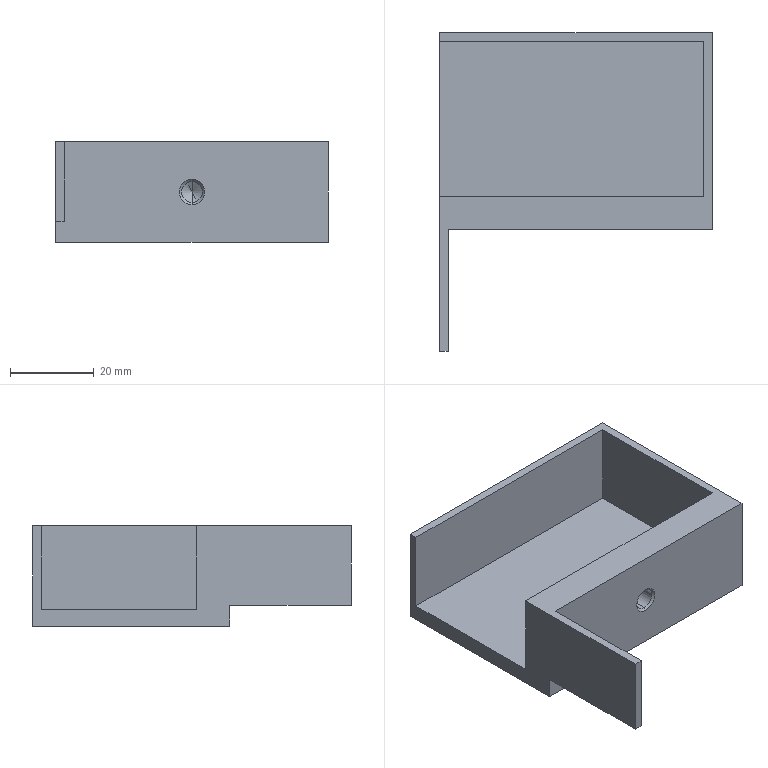Part | STEP file | 料槽1 | 1 solid | 19 faces | box 65 x 76 x 24 mm | volume 27672 mm3 | plane 13 | cone 4 | cylinder 2 | commonest cylinder face diameters 5 x2
STEP:
#1=CARTESIAN_POINT('',(159.5,-0.975,14.5));
#2=VERTEX_POINT('',#1);
#3=CARTESIAN_POINT('',(159.5,-0.975,9.5));
#4=VERTEX_POINT('',#3);
#5=CARTESIAN_POINT('',(159.5,-0.975,12.));
#6=DIRECTION('',(0.,-1.,0.));
#7=DIRECTION('',(0.,0.,-1.));
#8=AXIS2_PLACEMENT_3D('',#5,#6,#7);
#9=CIRCLE('',#8,2.5);
#10=EDGE_CURVE('',#2,#4,#9,.T.);
#11=ORIENTED_EDGE('',*,*,#10,.F.);
#12=CARTESIAN_POINT('',(159.5,-1.5,15.025));
#13=VERTEX_POINT('',#12);
#14=CARTESIAN_POINT('',(159.5,-1.5,15.025));
#15=DIRECTION('',(0.,-0.7071,0.7071));
#16=VECTOR('',#15,1000.);
#17=LINE('',#14,#16);
#18=EDGE_CURVE('',#2,#13,#17,.T.);
#19=ORIENTED_EDGE('',*,*,#18,.T.);
#20=CARTESIAN_POINT('',(159.5,-1.5,8.975));
#21=VERTEX_POINT('',#20);
#22=CARTESIAN_POINT('',(159.5,-1.5,12.));
#23=DIRECTION('',(0.,-1.,0.));
#24=DIRECTION('',(0.,0.,-1.));
#25=AXIS2_PLACEMENT_3D('',#22,#23,#24);
#26=CIRCLE('',#25,3.025);
#27=EDGE_CURVE('',#13,#21,#26,.T.);
#28=ORIENTED_EDGE('',*,*,#27,.T.);
#29=CARTESIAN_POINT('',(159.5,-1.5,8.975));
#30=DIRECTION('',(0.,-0.7071,-0.7071));
#31=VECTOR('',#30,1000.);
#32=LINE('',#29,#31);
#33=EDGE_CURVE('',#4,#21,#32,.T.);
#34=ORIENTED_EDGE('',*,*,#33,.F.);
#35=EDGE_LOOP('',(#11,#19,#28,#34));
#36=FACE_OUTER_BOUND('',#35,.T.);
#37=CARTESIAN_POINT('',(159.5,-1.5,12.));
#38=DIRECTION('',(0.,-1.,0.));
#39=DIRECTION('',(0.,0.,-1.));
#40=AXIS2_PLACEMENT_3D('',#37,#38,#39);
#41=CONICAL_SURFACE('',#40,3.025,0.7854);
#42=ADVANCED_FACE('',(#36),#41,.F.);
#43=CARTESIAN_POINT('',(159.5,4.5,14.5));
#44=VERTEX_POINT('',#43);
#45=CARTESIAN_POINT('',(159.5,4.5,9.5));
#46=VERTEX_POINT('',#45);
#47=CARTESIAN_POINT('',(159.5,4.5,12.));
#48=DIRECTION('',(0.,-1.,0.));
#49=DIRECTION('',(0.,0.,-1.));
#50=AXIS2_PLACEMENT_3D('',#47,#48,#49);
#51=CIRCLE('',#50,2.5);
#52=EDGE_CURVE('',#44,#46,#51,.T.);
#53=ORIENTED_EDGE('',*,*,#52,.F.);
#54=CARTESIAN_POINT('',(159.5,-1.5,14.5));
#55=DIRECTION('',(0.,-1.,0.));
#56=VECTOR('',#55,1000.);
#57=LINE('',#54,#56);
#58=EDGE_CURVE('',#44,#2,#57,.T.);
#59=ORIENTED_EDGE('',*,*,#58,.T.);
#60=ORIENTED_EDGE('',*,*,#10,.T.);
#61=CARTESIAN_POINT('',(159.5,-1.5,9.5));
#62=DIRECTION('',(0.,-1.,0.));
#63=VECTOR('',#62,1000.);
#64=LINE('',#61,#63);
#65=EDGE_CURVE('',#46,#4,#64,.T.);
#66=ORIENTED_EDGE('',*,*,#65,.F.);
#67=EDGE_LOOP('',(#53,#59,#60,#66));
#68=FACE_OUTER_BOUND('',#67,.T.);
#69=CARTESIAN_POINT('',(159.5,-1.5,12.));
#70=DIRECTION('',(0.,-1.,0.));
#71=DIRECTION('',(0.,0.,-1.));
#72=AXIS2_PLACEMENT_3D('',#69,#70,#71);
#73=CYLINDRICAL_SURFACE('',#72,2.5);
#74=ADVANCED_FACE('',(#68),#73,.F.);
#75=CARTESIAN_POINT('',(159.5,6.002,12.));
#76=VERTEX_POINT('',#75);
#77=CARTESIAN_POINT('',(159.5,4.5,9.5));
#78=DIRECTION('',(0.,-0.515,-0.8572));
#79=VECTOR('',#78,1000.);
#80=LINE('',#77,#79);
#81=EDGE_CURVE('',#76,#46,#80,.T.);
#82=ORIENTED_EDGE('',*,*,#81,.F.);
#83=CARTESIAN_POINT('',(159.5,4.5,14.5));
#84=DIRECTION('',(0.,-0.515,0.8572));
#85=VECTOR('',#84,1000.);
#86=LINE('',#83,#85);
#87=EDGE_CURVE('',#76,#44,#86,.T.);
#88=ORIENTED_EDGE('',*,*,#87,.T.);
#89=ORIENTED_EDGE('',*,*,#52,.T.);
#90=EDGE_LOOP('',(#82,#88,#89));
#91=FACE_OUTER_BOUND('',#90,.T.);
#92=CARTESIAN_POINT('',(159.5,4.5,12.));
#93=DIRECTION('',(0.,-1.,0.));
#94=DIRECTION('',(0.,0.,-1.));
#95=AXIS2_PLACEMENT_3D('',#92,#93,#94);
#96=CONICAL_SURFACE('',#95,2.5,1.03);
#97=ADVANCED_FACE('',(#91),#96,.F.);
#98=CARTESIAN_POINT('',(192.,45.5,0.));
#99=VERTEX_POINT('',#98);
#100=CARTESIAN_POINT('',(127.,45.5,0.));
#101=VERTEX_POINT('',#100);
#102=CARTESIAN_POINT('',(190.,45.5,0.));
#103=DIRECTION('',(-1.,0.,0.));
#104=VECTOR('',#103,1000.);
#105=LINE('',#102,#104);
#106=EDGE_CURVE('',#99,#101,#105,.T.);
#107=ORIENTED_EDGE('',*,*,#106,.T.);
#108=CARTESIAN_POINT('',(127.,45.5,24.));
#109=VERTEX_POINT('',#108);
#110=CARTESIAN_POINT('',(127.,45.5,4.));
#111=DIRECTION('',(0.,0.,-1.));
#112=VECTOR('',#111,1000.);
#113=LINE('',#110,#112);
#114=EDGE_CURVE('',#109,#101,#113,.T.);
#115=ORIENTED_EDGE('',*,*,#114,.F.);
#116=CARTESIAN_POINT('',(192.,45.5,24.));
#117=VERTEX_POINT('',#116);
#118=CARTESIAN_POINT('',(210.1,45.5,24.));
#119=DIRECTION('',(-1.,0.,0.));
#120=VECTOR('',#119,1000.);
#121=LINE('',#118,#120);
#122=EDGE_CURVE('',#117,#109,#121,.T.);
#123=ORIENTED_EDGE('',*,*,#122,.F.);
#124=CARTESIAN_POINT('',(192.,45.5,24.));
#125=DIRECTION('',(0.,0.,1.));
#126=VECTOR('',#125,1000.);
#127=LINE('',#124,#126);
#128=EDGE_CURVE('',#99,#117,#127,.T.);
#129=ORIENTED_EDGE('',*,*,#128,.F.);
#130=EDGE_LOOP('',(#107,#115,#123,#129));
#131=FACE_OUTER_BOUND('',#130,.T.);
#132=CARTESIAN_POINT('',(190.,45.5,4.));
#133=DIRECTION('',(0.,-1.,0.));
#134=DIRECTION('',(1.,0.,0.));
#135=AXIS2_PLACEMENT_3D('',#132,#133,#134);
#136=PLANE('',#135);
#137=ADVANCED_FACE('',(#131),#136,.F.);
#138=CARTESIAN_POINT('',(127.,-1.5,0.));
#139=VERTEX_POINT('',#138);
#140=CARTESIAN_POINT('',(127.,45.5,0.));
#141=DIRECTION('',(0.,-1.,0.));
#142=VECTOR('',#141,1000.);
#143=LINE('',#140,#142);
#144=EDGE_CURVE('',#101,#139,#143,.T.);
#145=ORIENTED_EDGE('',*,*,#144,.T.);
#146=CARTESIAN_POINT('',(127.,-1.5,5.));
#147=VERTEX_POINT('',#146);
#148=CARTESIAN_POINT('',(127.,-1.5,24.));
#149=DIRECTION('',(0.,0.,-1.));
#150=VECTOR('',#149,1000.);
#151=LINE('',#148,#150);
#152=EDGE_CURVE('',#147,#139,#151,.T.);
#153=ORIENTED_EDGE('',*,*,#152,.F.);
#154=CARTESIAN_POINT('',(127.,-30.5,5.));
#155=VERTEX_POINT('',#154);
#156=CARTESIAN_POINT('',(127.,-30.5,5.));
#157=DIRECTION('',(0.,1.,0.));
#158=VECTOR('',#157,1000.);
#159=LINE('',#156,#158);
#160=EDGE_CURVE('',#155,#147,#159,.T.);
#161=ORIENTED_EDGE('',*,*,#160,.F.);
#162=CARTESIAN_POINT('',(127.,-30.5,24.));
#163=VERTEX_POINT('',#162);
#164=CARTESIAN_POINT('',(127.,-30.5,24.));
#165=DIRECTION('',(0.,0.,-1.));
#166=VECTOR('',#165,1000.);
#167=LINE('',#164,#166);
#168=EDGE_CURVE('',#163,#155,#167,.T.);
#169=ORIENTED_EDGE('',*,*,#168,.F.);
#170=CARTESIAN_POINT('',(127.,6.5,24.));
#171=VERTEX_POINT('',#170);
#172=CARTESIAN_POINT('',(127.,4.5,24.));
#173=DIRECTION('',(0.,1.,0.));
#174=VECTOR('',#173,1000.);
#175=LINE('',#172,#174);
#176=EDGE_CURVE('',#163,#171,#175,.T.);
#177=ORIENTED_EDGE('',*,*,#176,.T.);
#178=CARTESIAN_POINT('',(127.,6.5,4.));
#179=VERTEX_POINT('',#178);
#180=CARTESIAN_POINT('',(127.,6.5,24.));
#181=DIRECTION('',(0.,0.,-1.));
#182=VECTOR('',#181,1000.);
#183=LINE('',#180,#182);
#184=EDGE_CURVE('',#171,#179,#183,.T.);
#185=ORIENTED_EDGE('',*,*,#184,.T.);
#186=CARTESIAN_POINT('',(127.,43.5,4.));
#187=VERTEX_POINT('',#186);
#188=CARTESIAN_POINT('',(127.,45.5,4.));
#189=DIRECTION('',(0.,-1.,0.));
#190=VECTOR('',#189,1000.);
#191=LINE('',#188,#190);
#192=EDGE_CURVE('',#187,#179,#191,.T.);
#193=ORIENTED_EDGE('',*,*,#192,.F.);
#194=CARTESIAN_POINT('',(127.,43.5,24.));
#195=VERTEX_POINT('',#194);
#196=CARTESIAN_POINT('',(127.,43.5,24.));
#197=DIRECTION('',(0.,0.,1.));
#198=VECTOR('',#197,1000.);
#199=LINE('',#196,#198);
#200=EDGE_CURVE('',#187,#195,#199,.T.);
#201=ORIENTED_EDGE('',*,*,#200,.T.);
#202=CARTESIAN_POINT('',(127.,45.5,24.));
#203=DIRECTION('',(0.,1.,0.));
#204=VECTOR('',#203,1000.);
#205=LINE('',#202,#204);
#206=EDGE_CURVE('',#195,#109,#205,.T.);
#207=ORIENTED_EDGE('',*,*,#206,.T.);
#208=ORIENTED_EDGE('',*,*,#114,.T.);
#209=EDGE_LOOP('',(#145,#153,#161,#169,#177,#185,#193,#201,#207,#208));
#210=FACE_OUTER_BOUND('',#209,.T.);
#211=CARTESIAN_POINT('',(127.,45.5,4.));
#212=DIRECTION('',(1.,0.,0.));
#213=DIRECTION('',(0.,0.,-1.));
#214=AXIS2_PLACEMENT_3D('',#211,#212,#213);
#215=PLANE('',#214);
#216=ADVANCED_FACE('',(#210),#215,.F.);
#217=ORIENTED_EDGE('',*,*,#192,.T.);
#218=CARTESIAN_POINT('',(190.,6.5,4.));
#219=VERTEX_POINT('',#218);
#220=CARTESIAN_POINT('',(210.1,6.5,4.));
#221=DIRECTION('',(-1.,0.,0.));
#222=VECTOR('',#221,1000.);
#223=LINE('',#220,#222);
#224=EDGE_CURVE('',#219,#179,#223,.T.);
#225=ORIENTED_EDGE('',*,*,#224,.F.);
#226=CARTESIAN_POINT('',(190.,43.5,4.));
#227=VERTEX_POINT('',#226);
#228=CARTESIAN_POINT('',(190.,45.5,4.));
#229=DIRECTION('',(0.,1.,0.));
#230=VECTOR('',#229,1000.);
#231=LINE('',#228,#230);
#232=EDGE_CURVE('',#219,#227,#231,.T.);
#233=ORIENTED_EDGE('',*,*,#232,.T.);
#234=CARTESIAN_POINT('',(210.1,43.5,4.));
#235=DIRECTION('',(-1.,0.,0.));
#236=VECTOR('',#235,1000.);
#237=LINE('',#234,#236);
#238=EDGE_CURVE('',#227,#187,#237,.T.);
#239=ORIENTED_EDGE('',*,*,#238,.T.);
#240=EDGE_LOOP('',(#217,#225,#233,#239));
#241=FACE_OUTER_BOUND('',#240,.T.);
#242=CARTESIAN_POINT('',(0.,0.,4.));
#243=DIRECTION('',(0.,0.,-1.));
#244=DIRECTION('',(-1.,0.,0.));
#245=AXIS2_PLACEMENT_3D('',#242,#243,#244);
#246=PLANE('',#245);
#247=ADVANCED_FACE('',(#241),#246,.F.);
#248=ORIENTED_EDGE('',*,*,#106,.F.);
#249=CARTESIAN_POINT('',(192.,-1.5,0.));
#250=VERTEX_POINT('',#249);
#251=CARTESIAN_POINT('',(192.,4.5,0.));
#252=DIRECTION('',(0.,1.,0.));
#253=VECTOR('',#252,1000.);
#254=LINE('',#251,#253);
#255=EDGE_CURVE('',#250,#99,#254,.T.);
#256=ORIENTED_EDGE('',*,*,#255,.F.);
#257=CARTESIAN_POINT('',(127.,-1.5,0.));
#258=DIRECTION('',(1.,0.,0.));
#259=VECTOR('',#258,1000.);
#260=LINE('',#257,#259);
#261=EDGE_CURVE('',#139,#250,#260,.T.);
#262=ORIENTED_EDGE('',*,*,#261,.F.);
#263=ORIENTED_EDGE('',*,*,#144,.F.);
#264=EDGE_LOOP('',(#248,#256,#262,#263));
#265=FACE_OUTER_BOUND('',#264,.T.);
#266=CARTESIAN_POINT('',(0.,0.,0.));
#267=DIRECTION('',(0.,0.,-1.));
#268=DIRECTION('',(-1.,0.,0.));
#269=AXIS2_PLACEMENT_3D('',#266,#267,#268);
#270=PLANE('',#269);
#271=ADVANCED_FACE('',(#265),#270,.T.);
#272=CARTESIAN_POINT('',(190.,43.5,24.));
#273=VERTEX_POINT('',#272);
#274=CARTESIAN_POINT('',(210.1,43.5,24.));
#275=DIRECTION('',(-1.,0.,0.));
#276=VECTOR('',#275,1000.);
#277=LINE('',#274,#276);
#278=EDGE_CURVE('',#273,#195,#277,.T.);
#279=ORIENTED_EDGE('',*,*,#278,.F.);
#280=CARTESIAN_POINT('',(190.,6.5,24.));
#281=VERTEX_POINT('',#280);
#282=CARTESIAN_POINT('',(190.,4.5,24.));
#283=DIRECTION('',(0.,-1.,0.));
#284=VECTOR('',#283,1000.);
#285=LINE('',#282,#284);
#286=EDGE_CURVE('',#273,#281,#285,.T.);
#287=ORIENTED_EDGE('',*,*,#286,.T.);
#288=CARTESIAN_POINT('',(210.1,6.5,24.));
#289=DIRECTION('',(-1.,0.,0.));
#290=VECTOR('',#289,1000.);
#291=LINE('',#288,#290);
#292=EDGE_CURVE('',#281,#171,#291,.T.);
#293=ORIENTED_EDGE('',*,*,#292,.T.);
#294=ORIENTED_EDGE('',*,*,#176,.F.);
#295=CARTESIAN_POINT('',(129.,-30.5,24.));
#296=VERTEX_POINT('',#295);
#297=CARTESIAN_POINT('',(127.,-30.5,24.));
#298=DIRECTION('',(-1.,0.,0.));
#299=VECTOR('',#298,1000.);
#300=LINE('',#297,#299);
#301=EDGE_CURVE('',#296,#163,#300,.T.);
#302=ORIENTED_EDGE('',*,*,#301,.F.);
#303=CARTESIAN_POINT('',(129.,-1.5,24.));
#304=VERTEX_POINT('',#303);
#305=CARTESIAN_POINT('',(129.,-30.5,24.));
#306=DIRECTION('',(0.,1.,0.));
#307=VECTOR('',#306,1000.);
#308=LINE('',#305,#307);
#309=EDGE_CURVE('',#296,#304,#308,.T.);
#310=ORIENTED_EDGE('',*,*,#309,.T.);
#311=CARTESIAN_POINT('',(192.,-1.5,24.));
#312=VERTEX_POINT('',#311);
#313=CARTESIAN_POINT('',(127.,-1.5,24.));
#314=DIRECTION('',(-1.,0.,0.));
#315=VECTOR('',#314,1000.);
#316=LINE('',#313,#315);
#317=EDGE_CURVE('',#312,#304,#316,.T.);
#318=ORIENTED_EDGE('',*,*,#317,.F.);
#319=CARTESIAN_POINT('',(192.,4.5,24.));
#320=DIRECTION('',(0.,-1.,0.));
#321=VECTOR('',#320,1000.);
#322=LINE('',#319,#321);
#323=EDGE_CURVE('',#117,#312,#322,.T.);
#324=ORIENTED_EDGE('',*,*,#323,.F.);
#325=ORIENTED_EDGE('',*,*,#122,.T.);
#326=ORIENTED_EDGE('',*,*,#206,.F.);
#327=EDGE_LOOP('',(#279,#287,#293,#294,#302,#310,#318,#324,#325,#326));
#328=FACE_OUTER_BOUND('',#327,.T.);
#329=CARTESIAN_POINT('',(210.1,45.5,24.));
#330=DIRECTION('',(0.,0.,1.));
#331=DIRECTION('',(1.,0.,0.));
#332=AXIS2_PLACEMENT_3D('',#329,#330,#331);
#333=PLANE('',#332);
#334=ADVANCED_FACE('',(#328),#333,.T.);
#335=CARTESIAN_POINT('',(190.,43.5,24.));
#336=DIRECTION('',(0.,0.,-1.));
#337=VECTOR('',#336,1000.);
#338=LINE('',#335,#337);
#339=EDGE_CURVE('',#273,#227,#338,.T.);
#340=ORIENTED_EDGE('',*,*,#339,.F.);
#341=ORIENTED_EDGE('',*,*,#278,.T.);
#342=ORIENTED_EDGE('',*,*,#200,.F.);
#343=ORIENTED_EDGE('',*,*,#238,.F.);
#344=EDGE_LOOP('',(#340,#341,#342,#343));
#345=FACE_OUTER_BOUND('',#344,.T.);
#346=CARTESIAN_POINT('',(210.1,43.5,24.));
#347=DIRECTION('',(0.,-1.,0.));
#348=DIRECTION('',(1.,0.,0.));
#349=AXIS2_PLACEMENT_3D('',#346,#347,#348);
#350=PLANE('',#349);
#351=ADVANCED_FACE('',(#345),#350,.T.);
#352=CARTESIAN_POINT('',(190.,6.5,24.));
#353=DIRECTION('',(0.,0.,1.));
#354=VECTOR('',#353,1000.);
#355=LINE('',#352,#354);
#356=EDGE_CURVE('',#219,#281,#355,.T.);
#357=ORIENTED_EDGE('',*,*,#356,.F.);
#358=ORIENTED_EDGE('',*,*,#224,.T.);
#359=ORIENTED_EDGE('',*,*,#184,.F.);
#360=ORIENTED_EDGE('',*,*,#292,.F.);
#361=EDGE_LOOP('',(#357,#358,#359,#360));
#362=FACE_OUTER_BOUND('',#361,.T.);
#363=CARTESIAN_POINT('',(210.1,6.5,24.));
#364=DIRECTION('',(0.,1.,0.));
#365=DIRECTION('',(-1.,0.,0.));
#366=AXIS2_PLACEMENT_3D('',#363,#364,#365);
#367=PLANE('',#366);
#368=ADVANCED_FACE('',(#362),#367,.T.);
#369=ORIENTED_EDGE('',*,*,#323,.T.);
#370=CARTESIAN_POINT('',(192.,-1.5,24.));
#371=DIRECTION('',(0.,0.,1.));
#372=VECTOR('',#371,1000.);
#373=LINE('',#370,#372);
#374=EDGE_CURVE('',#250,#312,#373,.T.);
#375=ORIENTED_EDGE('',*,*,#374,.F.);
#376=ORIENTED_EDGE('',*,*,#255,.T.);
#377=ORIENTED_EDGE('',*,*,#128,.T.);
#378=EDGE_LOOP('',(#369,#375,#376,#377));
#379=FACE_OUTER_BOUND('',#378,.T.);
#380=CARTESIAN_POINT('',(192.,0.,0.));
#381=DIRECTION('',(-1.,0.,0.));
#382=DIRECTION('',(0.,0.,1.));
#383=AXIS2_PLACEMENT_3D('',#380,#381,#382);
#384=PLANE('',#383);
#385=ADVANCED_FACE('',(#379),#384,.F.);
#386=ORIENTED_EDGE('',*,*,#286,.F.);
#387=ORIENTED_EDGE('',*,*,#339,.T.);
#388=ORIENTED_EDGE('',*,*,#232,.F.);
#389=ORIENTED_EDGE('',*,*,#356,.T.);
#390=EDGE_LOOP('',(#386,#387,#388,#389));
#391=FACE_OUTER_BOUND('',#390,.T.);
#392=CARTESIAN_POINT('',(190.,0.,0.));
#393=DIRECTION('',(-1.,0.,0.));
#394=DIRECTION('',(0.,0.,1.));
#395=AXIS2_PLACEMENT_3D('',#392,#393,#394);
#396=PLANE('',#395);
#397=ADVANCED_FACE('',(#391),#396,.T.);
#398=CARTESIAN_POINT('',(159.5,-1.5,12.));
#399=DIRECTION('',(0.,-1.,0.));
#400=DIRECTION('',(0.,0.,-1.));
#401=AXIS2_PLACEMENT_3D('',#398,#399,#400);
#402=CIRCLE('',#401,3.025);
#403=EDGE_CURVE('',#21,#13,#402,.T.);
#404=ORIENTED_EDGE('',*,*,#403,.F.);
#405=ORIENTED_EDGE('',*,*,#27,.F.);
#406=EDGE_LOOP('',(#404,#405));
#407=FACE_BOUND('',#406,.T.);
#408=CARTESIAN_POINT('',(129.,-1.5,5.));
#409=VERTEX_POINT('',#408);
#410=CARTESIAN_POINT('',(129.,-1.5,24.));
#411=DIRECTION('',(0.,0.,1.));
#412=VECTOR('',#411,1000.);
#413=LINE('',#410,#412);
#414=EDGE_CURVE('',#409,#304,#413,.T.);
#415=ORIENTED_EDGE('',*,*,#414,.F.);
#416=CARTESIAN_POINT('',(127.,-1.5,5.));
#417=DIRECTION('',(1.,0.,0.));
#418=VECTOR('',#417,1000.);
#419=LINE('',#416,#418);
#420=EDGE_CURVE('',#147,#409,#419,.T.);
#421=ORIENTED_EDGE('',*,*,#420,.F.);
#422=ORIENTED_EDGE('',*,*,#152,.T.);
#423=ORIENTED_EDGE('',*,*,#261,.T.);
#424=ORIENTED_EDGE('',*,*,#374,.T.);
#425=ORIENTED_EDGE('',*,*,#317,.T.);
#426=EDGE_LOOP('',(#415,#421,#422,#423,#424,#425));
#427=FACE_OUTER_BOUND('',#426,.T.);
#428=CARTESIAN_POINT('',(0.,-1.5,0.));
#429=DIRECTION('',(0.,-1.,0.));
#430=DIRECTION('',(1.,0.,0.));
#431=AXIS2_PLACEMENT_3D('',#428,#429,#430);
#432=PLANE('',#431);
#433=ADVANCED_FACE('',(#407,#427),#432,.T.);
#434=ORIENTED_EDGE('',*,*,#420,.T.);
#435=CARTESIAN_POINT('',(129.,-30.5,5.));
#436=VERTEX_POINT('',#435);
#437=CARTESIAN_POINT('',(129.,-30.5,5.));
#438=DIRECTION('',(0.,1.,0.));
#439=VECTOR('',#438,1000.);
#440=LINE('',#437,#439);
#441=EDGE_CURVE('',#436,#409,#440,.T.);
#442=ORIENTED_EDGE('',*,*,#441,.F.);
#443=CARTESIAN_POINT('',(127.,-30.5,5.));
#444=DIRECTION('',(1.,0.,0.));
#445=VECTOR('',#444,1000.);
#446=LINE('',#443,#445);
#447=EDGE_CURVE('',#155,#436,#446,.T.);
#448=ORIENTED_EDGE('',*,*,#447,.F.);
#449=ORIENTED_EDGE('',*,*,#160,.T.);
#450=EDGE_LOOP('',(#434,#442,#448,#449));
#451=FACE_OUTER_BOUND('',#450,.T.);
#452=CARTESIAN_POINT('',(127.,-30.5,5.));
#453=DIRECTION('',(0.,0.,1.));
#454=DIRECTION('',(1.,0.,0.));
#455=AXIS2_PLACEMENT_3D('',#452,#453,#454);
#456=PLANE('',#455);
#457=ADVANCED_FACE('',(#451),#456,.F.);
#458=ORIENTED_EDGE('',*,*,#414,.T.);
#459=ORIENTED_EDGE('',*,*,#309,.F.);
#460=CARTESIAN_POINT('',(129.,-30.5,24.));
#461=DIRECTION('',(0.,0.,1.));
#462=VECTOR('',#461,1000.);
#463=LINE('',#460,#462);
#464=EDGE_CURVE('',#436,#296,#463,.T.);
#465=ORIENTED_EDGE('',*,*,#464,.F.);
#466=ORIENTED_EDGE('',*,*,#441,.T.);
#467=EDGE_LOOP('',(#458,#459,#465,#466));
#468=FACE_OUTER_BOUND('',#467,.T.);
#469=CARTESIAN_POINT('',(129.,-30.5,24.));
#470=DIRECTION('',(-1.,0.,0.));
#471=DIRECTION('',(0.,-1.,0.));
#472=AXIS2_PLACEMENT_3D('',#469,#470,#471);
#473=PLANE('',#472);
#474=ADVANCED_FACE('',(#468),#473,.F.);
#475=ORIENTED_EDGE('',*,*,#168,.T.);
#476=ORIENTED_EDGE('',*,*,#447,.T.);
#477=ORIENTED_EDGE('',*,*,#464,.T.);
#478=ORIENTED_EDGE('',*,*,#301,.T.);
#479=EDGE_LOOP('',(#475,#476,#477,#478));
#480=FACE_OUTER_BOUND('',#479,.T.);
#481=CARTESIAN_POINT('',(0.,-30.5,0.));
#482=DIRECTION('',(0.,-1.,0.));
#483=DIRECTION('',(1.,0.,0.));
#484=AXIS2_PLACEMENT_3D('',#481,#482,#483);
#485=PLANE('',#484);
#486=ADVANCED_FACE('',(#480),#485,.T.);
#487=ORIENTED_EDGE('',*,*,#87,.F.);
#488=ORIENTED_EDGE('',*,*,#81,.T.);
#489=CARTESIAN_POINT('',(159.5,4.5,12.));
#490=DIRECTION('',(0.,-1.,0.));
#491=DIRECTION('',(0.,0.,-1.));
#492=AXIS2_PLACEMENT_3D('',#489,#490,#491);
#493=CIRCLE('',#492,2.5);
#494=EDGE_CURVE('',#46,#44,#493,.T.);
#495=ORIENTED_EDGE('',*,*,#494,.T.);
#496=EDGE_LOOP('',(#487,#488,#495));
#497=FACE_OUTER_BOUND('',#496,.T.);
#498=CARTESIAN_POINT('',(159.5,4.5,12.));
#499=DIRECTION('',(0.,-1.,0.));
#500=DIRECTION('',(0.,0.,-1.));
#501=AXIS2_PLACEMENT_3D('',#498,#499,#500);
#502=CONICAL_SURFACE('',#501,2.5,1.03);
#503=ADVANCED_FACE('',(#497),#502,.F.);
#504=ORIENTED_EDGE('',*,*,#58,.F.);
#505=ORIENTED_EDGE('',*,*,#494,.F.);
#506=ORIENTED_EDGE('',*,*,#65,.T.);
#507=CARTESIAN_POINT('',(159.5,-0.975,12.));
#508=DIRECTION('',(0.,-1.,0.));
#509=DIRECTION('',(0.,0.,-1.));
#510=AXIS2_PLACEMENT_3D('',#507,#508,#509);
#511=CIRCLE('',#510,2.5);
#512=EDGE_CURVE('',#4,#2,#511,.T.);
#513=ORIENTED_EDGE('',*,*,#512,.T.);
#514=EDGE_LOOP('',(#504,#505,#506,#513));
#515=FACE_OUTER_BOUND('',#514,.T.);
#516=CARTESIAN_POINT('',(159.5,-1.5,12.));
#517=DIRECTION('',(0.,-1.,0.));
#518=DIRECTION('',(0.,0.,-1.));
#519=AXIS2_PLACEMENT_3D('',#516,#517,#518);
#520=CYLINDRICAL_SURFACE('',#519,2.5);
#521=ADVANCED_FACE('',(#515),#520,.F.);
#522=ORIENTED_EDGE('',*,*,#18,.F.);
#523=ORIENTED_EDGE('',*,*,#512,.F.);
#524=ORIENTED_EDGE('',*,*,#33,.T.);
#525=ORIENTED_EDGE('',*,*,#403,.T.);
#526=EDGE_LOOP('',(#522,#523,#524,#525));
#527=FACE_OUTER_BOUND('',#526,.T.);
#528=CARTESIAN_POINT('',(159.5,-1.5,12.));
#529=DIRECTION('',(0.,-1.,0.));
#530=DIRECTION('',(0.,0.,-1.));
#531=AXIS2_PLACEMENT_3D('',#528,#529,#530);
#532=CONICAL_SURFACE('',#531,3.025,0.7854);
#533=ADVANCED_FACE('',(#527),#532,.F.);
#534=CLOSED_SHELL('',(#42,#74,#97,#137,#216,#247,#271,#334,#351,#368,#385,#397,#433,#457,#474,#486,#503,#521,#533));
#535=MANIFOLD_SOLID_BREP('',#534);
#536=CARTESIAN_POINT('',(0.,0.,0.));
#537=DIRECTION('',(0.,0.,1.));
#538=DIRECTION('',(1.,0.,0.));
#539=AXIS2_PLACEMENT_3D('',#536,#537,#538);
#540=(LENGTH_UNIT()NAMED_UNIT(*)SI_UNIT(.MILLI.,.METRE.));
#541=UNCERTAINTY_MEASURE_WITH_UNIT(LENGTH_MEASURE(0.00001),#540,'','');
#542=(NAMED_UNIT(*)PLANE_ANGLE_UNIT()SI_UNIT($,.RADIAN.));
#543=(NAMED_UNIT(*)SI_UNIT($,.STERADIAN.)SOLID_ANGLE_UNIT());
#544=(GEOMETRIC_REPRESENTATION_CONTEXT(3)GLOBAL_UNCERTAINTY_ASSIGNED_CONTEXT((#541))GLOBAL_UNIT_ASSIGNED_CONTEXT((#540,#542,#543))REPRESENTATION_CONTEXT('',''));
#545=ADVANCED_BREP_SHAPE_REPRESENTATION('',(#535,#539),#544);